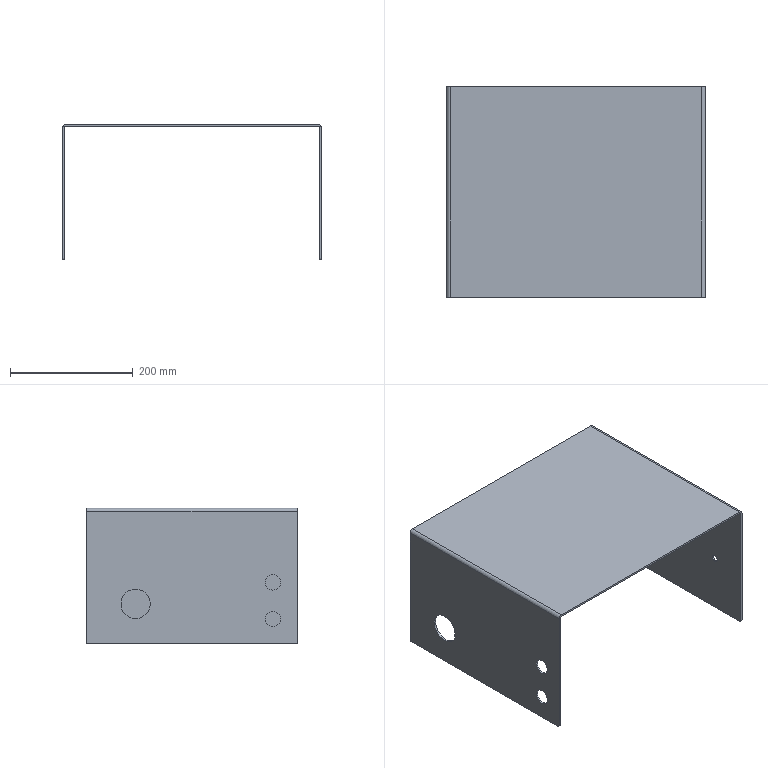Part | SolidWorks | features ICE 2, Fillet 1, FlatPattern 1, SMBaseFlange 1, SheetMetal 1, UnFold 1 | 1 solid | 36 faces | box 422 x 344 x 221 mm | volume 872945 mm3 | cylinder 18 | plane 18 | commonest cylinder face diameters 11 x6 6 x4 25 x4 5 x2 48 x2
STEP:
#1=CARTESIAN_POINT('',(-208.,92.,-180.));
#2=VERTEX_POINT('',#1);
#3=CARTESIAN_POINT('',(-208.,92.,-132.));
#4=VERTEX_POINT('',#3);
#5=CARTESIAN_POINT('',(-208.,92.,-156.));
#6=DIRECTION('',(-1.,0.,0.));
#7=DIRECTION('',(0.,0.,1.));
#8=AXIS2_PLACEMENT_3D('',#5,#6,#7);
#9=CIRCLE('',#8,24.);
#10=EDGE_CURVE('',#2,#4,#9,.T.);
#11=ORIENTED_EDGE('',*,*,#10,.F.);
#12=CARTESIAN_POINT('',(-211.,92.,-180.));
#13=VERTEX_POINT('',#12);
#14=CARTESIAN_POINT('',(-208.,92.,-180.));
#15=DIRECTION('',(-1.,0.,0.));
#16=VECTOR('',#15,1000.);
#17=LINE('',#14,#16);
#18=EDGE_CURVE('',#2,#13,#17,.T.);
#19=ORIENTED_EDGE('',*,*,#18,.T.);
#20=CARTESIAN_POINT('',(-211.,92.,-132.));
#21=VERTEX_POINT('',#20);
#22=CARTESIAN_POINT('',(-211.,92.,-156.));
#23=DIRECTION('',(-1.,0.,0.));
#24=DIRECTION('',(0.,0.,1.));
#25=AXIS2_PLACEMENT_3D('',#22,#23,#24);
#26=CIRCLE('',#25,24.);
#27=EDGE_CURVE('',#13,#21,#26,.T.);
#28=ORIENTED_EDGE('',*,*,#27,.T.);
#29=CARTESIAN_POINT('',(-208.,92.,-132.));
#30=DIRECTION('',(-1.,0.,0.));
#31=VECTOR('',#30,1000.);
#32=LINE('',#29,#31);
#33=EDGE_CURVE('',#4,#21,#32,.T.);
#34=ORIENTED_EDGE('',*,*,#33,.F.);
#35=EDGE_LOOP('',(#11,#19,#28,#34));
#36=FACE_OUTER_BOUND('',#35,.T.);
#37=CARTESIAN_POINT('',(-208.,92.,-156.));
#38=DIRECTION('',(-1.,0.,0.));
#39=DIRECTION('',(0.,0.,1.));
#40=AXIS2_PLACEMENT_3D('',#37,#38,#39);
#41=CYLINDRICAL_SURFACE('',#40,24.);
#42=ADVANCED_FACE('',(#36),#41,.F.);
#43=CARTESIAN_POINT('',(-208.,-132.,-193.5));
#44=VERTEX_POINT('',#43);
#45=CARTESIAN_POINT('',(-208.,-132.,-168.5));
#46=VERTEX_POINT('',#45);
#47=CARTESIAN_POINT('',(-208.,-132.,-181.));
#48=DIRECTION('',(-1.,0.,0.));
#49=DIRECTION('',(0.,0.,1.));
#50=AXIS2_PLACEMENT_3D('',#47,#48,#49);
#51=CIRCLE('',#50,12.5);
#52=EDGE_CURVE('',#44,#46,#51,.T.);
#53=ORIENTED_EDGE('',*,*,#52,.F.);
#54=CARTESIAN_POINT('',(-211.,-132.,-193.5));
#55=VERTEX_POINT('',#54);
#56=CARTESIAN_POINT('',(-208.,-132.,-193.5));
#57=DIRECTION('',(-1.,0.,0.));
#58=VECTOR('',#57,1000.);
#59=LINE('',#56,#58);
#60=EDGE_CURVE('',#44,#55,#59,.T.);
#61=ORIENTED_EDGE('',*,*,#60,.T.);
#62=CARTESIAN_POINT('',(-211.,-132.,-168.5));
#63=VERTEX_POINT('',#62);
#64=CARTESIAN_POINT('',(-211.,-132.,-181.));
#65=DIRECTION('',(-1.,0.,0.));
#66=DIRECTION('',(0.,0.,1.));
#67=AXIS2_PLACEMENT_3D('',#64,#65,#66);
#68=CIRCLE('',#67,12.5);
#69=EDGE_CURVE('',#55,#63,#68,.T.);
#70=ORIENTED_EDGE('',*,*,#69,.T.);
#71=CARTESIAN_POINT('',(-208.,-132.,-168.5));
#72=DIRECTION('',(-1.,0.,0.));
#73=VECTOR('',#72,1000.);
#74=LINE('',#71,#73);
#75=EDGE_CURVE('',#46,#63,#74,.T.);
#76=ORIENTED_EDGE('',*,*,#75,.F.);
#77=EDGE_LOOP('',(#53,#61,#70,#76));
#78=FACE_OUTER_BOUND('',#77,.T.);
#79=CARTESIAN_POINT('',(-208.,-132.,-181.));
#80=DIRECTION('',(-1.,0.,0.));
#81=DIRECTION('',(0.,0.,1.));
#82=AXIS2_PLACEMENT_3D('',#79,#80,#81);
#83=CYLINDRICAL_SURFACE('',#82,12.5);
#84=ADVANCED_FACE('',(#78),#83,.F.);
#85=CARTESIAN_POINT('',(-208.,-132.,-133.5));
#86=VERTEX_POINT('',#85);
#87=CARTESIAN_POINT('',(-208.,-132.,-108.5));
#88=VERTEX_POINT('',#87);
#89=CARTESIAN_POINT('',(-208.,-132.,-121.));
#90=DIRECTION('',(-1.,0.,0.));
#91=DIRECTION('',(0.,0.,1.));
#92=AXIS2_PLACEMENT_3D('',#89,#90,#91);
#93=CIRCLE('',#92,12.5);
#94=EDGE_CURVE('',#86,#88,#93,.T.);
#95=ORIENTED_EDGE('',*,*,#94,.F.);
#96=CARTESIAN_POINT('',(-211.,-132.,-133.5));
#97=VERTEX_POINT('',#96);
#98=CARTESIAN_POINT('',(-208.,-132.,-133.5));
#99=DIRECTION('',(-1.,0.,0.));
#100=VECTOR('',#99,1000.);
#101=LINE('',#98,#100);
#102=EDGE_CURVE('',#86,#97,#101,.T.);
#103=ORIENTED_EDGE('',*,*,#102,.T.);
#104=CARTESIAN_POINT('',(-211.,-132.,-108.5));
#105=VERTEX_POINT('',#104);
#106=CARTESIAN_POINT('',(-211.,-132.,-121.));
#107=DIRECTION('',(-1.,0.,0.));
#108=DIRECTION('',(0.,0.,1.));
#109=AXIS2_PLACEMENT_3D('',#106,#107,#108);
#110=CIRCLE('',#109,12.5);
#111=EDGE_CURVE('',#97,#105,#110,.T.);
#112=ORIENTED_EDGE('',*,*,#111,.T.);
#113=CARTESIAN_POINT('',(-208.,-132.,-108.5));
#114=DIRECTION('',(-1.,0.,0.));
#115=VECTOR('',#114,1000.);
#116=LINE('',#113,#115);
#117=EDGE_CURVE('',#88,#105,#116,.T.);
#118=ORIENTED_EDGE('',*,*,#117,.F.);
#119=EDGE_LOOP('',(#95,#103,#112,#118));
#120=FACE_OUTER_BOUND('',#119,.T.);
#121=CARTESIAN_POINT('',(-208.,-132.,-121.));
#122=DIRECTION('',(-1.,0.,0.));
#123=DIRECTION('',(0.,0.,1.));
#124=AXIS2_PLACEMENT_3D('',#121,#122,#123);
#125=CYLINDRICAL_SURFACE('',#124,12.5);
#126=ADVANCED_FACE('',(#120),#125,.F.);
#127=CARTESIAN_POINT('',(208.,-112.,-118.5));
#128=VERTEX_POINT('',#127);
#129=CARTESIAN_POINT('',(208.,-112.,-129.5));
#130=VERTEX_POINT('',#129);
#131=CARTESIAN_POINT('',(208.,-112.,-124.));
#132=DIRECTION('',(1.,0.,0.));
#133=DIRECTION('',(0.,0.,-1.));
#134=AXIS2_PLACEMENT_3D('',#131,#132,#133);
#135=CIRCLE('',#134,5.5);
#136=EDGE_CURVE('',#128,#130,#135,.T.);
#137=ORIENTED_EDGE('',*,*,#136,.F.);
#138=CARTESIAN_POINT('',(211.,-112.,-118.5));
#139=VERTEX_POINT('',#138);
#140=CARTESIAN_POINT('',(208.,-112.,-118.5));
#141=DIRECTION('',(1.,0.,0.));
#142=VECTOR('',#141,1000.);
#143=LINE('',#140,#142);
#144=EDGE_CURVE('',#128,#139,#143,.T.);
#145=ORIENTED_EDGE('',*,*,#144,.T.);
#146=CARTESIAN_POINT('',(211.,-112.,-129.5));
#147=VERTEX_POINT('',#146);
#148=CARTESIAN_POINT('',(211.,-112.,-124.));
#149=DIRECTION('',(1.,0.,0.));
#150=DIRECTION('',(0.,0.,-1.));
#151=AXIS2_PLACEMENT_3D('',#148,#149,#150);
#152=CIRCLE('',#151,5.5);
#153=EDGE_CURVE('',#139,#147,#152,.T.);
#154=ORIENTED_EDGE('',*,*,#153,.T.);
#155=CARTESIAN_POINT('',(208.,-112.,-129.5));
#156=DIRECTION('',(1.,0.,0.));
#157=VECTOR('',#156,1000.);
#158=LINE('',#155,#157);
#159=EDGE_CURVE('',#130,#147,#158,.T.);
#160=ORIENTED_EDGE('',*,*,#159,.F.);
#161=EDGE_LOOP('',(#137,#145,#154,#160));
#162=FACE_OUTER_BOUND('',#161,.T.);
#163=CARTESIAN_POINT('',(208.,-112.,-124.));
#164=DIRECTION('',(1.,0.,0.));
#165=DIRECTION('',(0.,0.,-1.));
#166=AXIS2_PLACEMENT_3D('',#163,#164,#165);
#167=CYLINDRICAL_SURFACE('',#166,5.5);
#168=ADVANCED_FACE('',(#162),#167,.F.);
#169=CARTESIAN_POINT('',(208.,38.,-118.5));
#170=VERTEX_POINT('',#169);
#171=CARTESIAN_POINT('',(208.,38.,-129.5));
#172=VERTEX_POINT('',#171);
#173=CARTESIAN_POINT('',(208.,38.,-124.));
#174=DIRECTION('',(1.,0.,0.));
#175=DIRECTION('',(0.,0.,-1.));
#176=AXIS2_PLACEMENT_3D('',#173,#174,#175);
#177=CIRCLE('',#176,5.5);
#178=EDGE_CURVE('',#170,#172,#177,.T.);
#179=ORIENTED_EDGE('',*,*,#178,.F.);
#180=CARTESIAN_POINT('',(211.,38.,-118.5));
#181=VERTEX_POINT('',#180);
#182=CARTESIAN_POINT('',(208.,38.,-118.5));
#183=DIRECTION('',(1.,0.,0.));
#184=VECTOR('',#183,1000.);
#185=LINE('',#182,#184);
#186=EDGE_CURVE('',#170,#181,#185,.T.);
#187=ORIENTED_EDGE('',*,*,#186,.T.);
#188=CARTESIAN_POINT('',(211.,38.,-129.5));
#189=VERTEX_POINT('',#188);
#190=CARTESIAN_POINT('',(211.,38.,-124.));
#191=DIRECTION('',(1.,0.,0.));
#192=DIRECTION('',(0.,0.,-1.));
#193=AXIS2_PLACEMENT_3D('',#190,#191,#192);
#194=CIRCLE('',#193,5.5);
#195=EDGE_CURVE('',#181,#189,#194,.T.);
#196=ORIENTED_EDGE('',*,*,#195,.T.);
#197=CARTESIAN_POINT('',(208.,38.,-129.5));
#198=DIRECTION('',(1.,0.,0.));
#199=VECTOR('',#198,1000.);
#200=LINE('',#197,#199);
#201=EDGE_CURVE('',#172,#189,#200,.T.);
#202=ORIENTED_EDGE('',*,*,#201,.F.);
#203=EDGE_LOOP('',(#179,#187,#196,#202));
#204=FACE_OUTER_BOUND('',#203,.T.);
#205=CARTESIAN_POINT('',(208.,38.,-124.));
#206=DIRECTION('',(1.,0.,0.));
#207=DIRECTION('',(0.,0.,-1.));
#208=AXIS2_PLACEMENT_3D('',#205,#206,#207);
#209=CYLINDRICAL_SURFACE('',#208,5.5);
#210=ADVANCED_FACE('',(#204),#209,.F.);
#211=CARTESIAN_POINT('',(205.5,172.,0.));
#212=VERTEX_POINT('',#211);
#213=CARTESIAN_POINT('',(205.5,172.,-3.));
#214=VERTEX_POINT('',#213);
#215=CARTESIAN_POINT('',(205.5,172.,0.));
#216=DIRECTION('',(0.,0.,-1.));
#217=VECTOR('',#216,1000.);
#218=LINE('',#215,#217);
#219=EDGE_CURVE('',#212,#214,#218,.T.);
#220=ORIENTED_EDGE('',*,*,#219,.F.);
#221=CARTESIAN_POINT('',(211.,172.,-5.5));
#222=VERTEX_POINT('',#221);
#223=CARTESIAN_POINT('',(205.5,172.,-5.5));
#224=DIRECTION('',(0.,-1.,0.));
#225=DIRECTION('',(0.,0.,1.));
#226=AXIS2_PLACEMENT_3D('',#223,#224,#225);
#227=CIRCLE('',#226,5.5);
#228=EDGE_CURVE('',#222,#212,#227,.T.);
#229=ORIENTED_EDGE('',*,*,#228,.F.);
#230=CARTESIAN_POINT('',(208.,172.,-5.5));
#231=VERTEX_POINT('',#230);
#232=CARTESIAN_POINT('',(208.,172.,-5.5));
#233=DIRECTION('',(1.,0.,0.));
#234=VECTOR('',#233,1000.);
#235=LINE('',#232,#234);
#236=EDGE_CURVE('',#231,#222,#235,.T.);
#237=ORIENTED_EDGE('',*,*,#236,.F.);
#238=CARTESIAN_POINT('',(205.5,172.,-5.5));
#239=DIRECTION('',(0.,-1.,0.));
#240=DIRECTION('',(1.,0.,0.));
#241=AXIS2_PLACEMENT_3D('',#238,#239,#240);
#242=CIRCLE('',#241,2.5);
#243=EDGE_CURVE('',#231,#214,#242,.T.);
#244=ORIENTED_EDGE('',*,*,#243,.T.);
#245=EDGE_LOOP('',(#220,#229,#237,#244));
#246=FACE_OUTER_BOUND('',#245,.T.);
#247=CARTESIAN_POINT('',(205.5,172.,0.));
#248=DIRECTION('',(0.,1.,0.));
#249=DIRECTION('',(0.,0.,1.));
#250=AXIS2_PLACEMENT_3D('',#247,#248,#249);
#251=PLANE('',#250);
#252=ADVANCED_FACE('',(#246),#251,.T.);
#253=CARTESIAN_POINT('',(-205.5,172.,0.));
#254=VERTEX_POINT('',#253);
#255=CARTESIAN_POINT('',(-211.,172.,0.));
#256=DIRECTION('',(-1.,0.,0.));
#257=VECTOR('',#256,1000.);
#258=LINE('',#255,#257);
#259=EDGE_CURVE('',#212,#254,#258,.T.);
#260=ORIENTED_EDGE('',*,*,#259,.F.);
#261=ORIENTED_EDGE('',*,*,#219,.T.);
#262=CARTESIAN_POINT('',(-205.5,172.,-3.));
#263=VERTEX_POINT('',#262);
#264=CARTESIAN_POINT('',(-211.,172.,-3.));
#265=DIRECTION('',(-1.,0.,0.));
#266=VECTOR('',#265,1000.);
#267=LINE('',#264,#266);
#268=EDGE_CURVE('',#214,#263,#267,.T.);
#269=ORIENTED_EDGE('',*,*,#268,.T.);
#270=CARTESIAN_POINT('',(-205.5,172.,-3.));
#271=DIRECTION('',(0.,0.,1.));
#272=VECTOR('',#271,1000.);
#273=LINE('',#270,#272);
#274=EDGE_CURVE('',#263,#254,#273,.T.);
#275=ORIENTED_EDGE('',*,*,#274,.T.);
#276=EDGE_LOOP('',(#260,#261,#269,#275));
#277=FACE_OUTER_BOUND('',#276,.T.);
#278=CARTESIAN_POINT('',(208.,172.,-5.5));
#279=DIRECTION('',(0.,1.,0.));
#280=DIRECTION('',(0.,0.,1.));
#281=AXIS2_PLACEMENT_3D('',#278,#279,#280);
#282=PLANE('',#281);
#283=ADVANCED_FACE('',(#277),#282,.T.);
#284=CARTESIAN_POINT('',(211.,-172.,-5.5));
#285=VERTEX_POINT('',#284);
#286=CARTESIAN_POINT('',(208.,-172.,-5.5));
#287=VERTEX_POINT('',#286);
#288=CARTESIAN_POINT('',(211.,-172.,-5.5));
#289=DIRECTION('',(-1.,0.,0.));
#290=VECTOR('',#289,1000.);
#291=LINE('',#288,#290);
#292=EDGE_CURVE('',#285,#287,#291,.T.);
#293=ORIENTED_EDGE('',*,*,#292,.F.);
#294=CARTESIAN_POINT('',(205.5,-172.,0.));
#295=VERTEX_POINT('',#294);
#296=CARTESIAN_POINT('',(205.5,-172.,-5.5));
#297=DIRECTION('',(0.,-1.,0.));
#298=DIRECTION('',(0.,0.,1.));
#299=AXIS2_PLACEMENT_3D('',#296,#297,#298);
#300=CIRCLE('',#299,5.5);
#301=EDGE_CURVE('',#285,#295,#300,.T.);
#302=ORIENTED_EDGE('',*,*,#301,.T.);
#303=CARTESIAN_POINT('',(205.5,-172.,-3.));
#304=VERTEX_POINT('',#303);
#305=CARTESIAN_POINT('',(205.5,-172.,-3.));
#306=DIRECTION('',(0.,0.,1.));
#307=VECTOR('',#306,1000.);
#308=LINE('',#305,#307);
#309=EDGE_CURVE('',#304,#295,#308,.T.);
#310=ORIENTED_EDGE('',*,*,#309,.F.);
#311=CARTESIAN_POINT('',(205.5,-172.,-5.5));
#312=DIRECTION('',(0.,-1.,0.));
#313=DIRECTION('',(1.,0.,0.));
#314=AXIS2_PLACEMENT_3D('',#311,#312,#313);
#315=CIRCLE('',#314,2.5);
#316=EDGE_CURVE('',#287,#304,#315,.T.);
#317=ORIENTED_EDGE('',*,*,#316,.F.);
#318=EDGE_LOOP('',(#293,#302,#310,#317));
#319=FACE_OUTER_BOUND('',#318,.T.);
#320=CARTESIAN_POINT('',(211.,-172.,-5.5));
#321=DIRECTION('',(0.,-1.,0.));
#322=DIRECTION('',(0.,0.,-1.));
#323=AXIS2_PLACEMENT_3D('',#320,#321,#322);
#324=PLANE('',#323);
#325=ADVANCED_FACE('',(#319),#324,.T.);
#326=CARTESIAN_POINT('',(208.,-172.,-218.));
#327=VERTEX_POINT('',#326);
#328=CARTESIAN_POINT('',(208.,-172.,0.));
#329=DIRECTION('',(0.,0.,1.));
#330=VECTOR('',#329,1000.);
#331=LINE('',#328,#330);
#332=EDGE_CURVE('',#327,#287,#331,.T.);
#333=ORIENTED_EDGE('',*,*,#332,.F.);
#334=CARTESIAN_POINT('',(211.,-172.,-218.));
#335=VERTEX_POINT('',#334);
#336=CARTESIAN_POINT('',(205.5,-172.,-218.));
#337=DIRECTION('',(1.,0.,0.));
#338=VECTOR('',#337,1000.);
#339=LINE('',#336,#338);
#340=EDGE_CURVE('',#327,#335,#339,.T.);
#341=ORIENTED_EDGE('',*,*,#340,.T.);
#342=CARTESIAN_POINT('',(211.,-172.,0.));
#343=DIRECTION('',(0.,0.,1.));
#344=VECTOR('',#343,1000.);
#345=LINE('',#342,#344);
#346=EDGE_CURVE('',#335,#285,#345,.T.);
#347=ORIENTED_EDGE('',*,*,#346,.T.);
#348=ORIENTED_EDGE('',*,*,#292,.T.);
#349=EDGE_LOOP('',(#333,#341,#347,#348));
#350=FACE_OUTER_BOUND('',#349,.T.);
#351=CARTESIAN_POINT('',(205.5,-172.,-3.));
#352=DIRECTION('',(0.,-1.,0.));
#353=DIRECTION('',(0.,0.,-1.));
#354=AXIS2_PLACEMENT_3D('',#351,#352,#353);
#355=PLANE('',#354);
#356=ADVANCED_FACE('',(#350),#355,.T.);
#357=CARTESIAN_POINT('',(-211.,172.,-5.5));
#358=VERTEX_POINT('',#357);
#359=CARTESIAN_POINT('',(-208.,172.,-5.5));
#360=VERTEX_POINT('',#359);
#361=CARTESIAN_POINT('',(-211.,172.,-5.5));
#362=DIRECTION('',(1.,0.,0.));
#363=VECTOR('',#362,1000.);
#364=LINE('',#361,#363);
#365=EDGE_CURVE('',#358,#360,#364,.T.);
#366=ORIENTED_EDGE('',*,*,#365,.F.);
#367=CARTESIAN_POINT('',(-205.5,172.,-5.5));
#368=DIRECTION('',(0.,-1.,0.));
#369=DIRECTION('',(0.,0.,1.));
#370=AXIS2_PLACEMENT_3D('',#367,#368,#369);
#371=CIRCLE('',#370,5.5);
#372=EDGE_CURVE('',#254,#358,#371,.T.);
#373=ORIENTED_EDGE('',*,*,#372,.F.);
#374=ORIENTED_EDGE('',*,*,#274,.F.);
#375=CARTESIAN_POINT('',(-205.5,172.,-5.5));
#376=DIRECTION('',(0.,-1.,0.));
#377=DIRECTION('',(1.,0.,0.));
#378=AXIS2_PLACEMENT_3D('',#375,#376,#377);
#379=CIRCLE('',#378,2.5);
#380=EDGE_CURVE('',#263,#360,#379,.T.);
#381=ORIENTED_EDGE('',*,*,#380,.T.);
#382=EDGE_LOOP('',(#366,#373,#374,#381));
#383=FACE_OUTER_BOUND('',#382,.T.);
#384=CARTESIAN_POINT('',(-211.,172.,-5.5));
#385=DIRECTION('',(0.,1.,0.));
#386=DIRECTION('',(0.,0.,1.));
#387=AXIS2_PLACEMENT_3D('',#384,#385,#386);
#388=PLANE('',#387);
#389=ADVANCED_FACE('',(#383),#388,.T.);
#390=CARTESIAN_POINT('',(-208.,172.,-218.));
#391=VERTEX_POINT('',#390);
#392=CARTESIAN_POINT('',(-208.,172.,0.));
#393=DIRECTION('',(0.,0.,-1.));
#394=VECTOR('',#393,1000.);
#395=LINE('',#392,#394);
#396=EDGE_CURVE('',#360,#391,#395,.T.);
#397=ORIENTED_EDGE('',*,*,#396,.T.);
#398=CARTESIAN_POINT('',(-211.,172.,-218.));
#399=VERTEX_POINT('',#398);
#400=CARTESIAN_POINT('',(-205.5,172.,-218.));
#401=DIRECTION('',(-1.,0.,0.));
#402=VECTOR('',#401,1000.);
#403=LINE('',#400,#402);
#404=EDGE_CURVE('',#391,#399,#403,.T.);
#405=ORIENTED_EDGE('',*,*,#404,.T.);
#406=CARTESIAN_POINT('',(-211.,172.,0.));
#407=DIRECTION('',(0.,0.,-1.));
#408=VECTOR('',#407,1000.);
#409=LINE('',#406,#408);
#410=EDGE_CURVE('',#358,#399,#409,.T.);
#411=ORIENTED_EDGE('',*,*,#410,.F.);
#412=ORIENTED_EDGE('',*,*,#365,.T.);
#413=EDGE_LOOP('',(#397,#405,#411,#412));
#414=FACE_OUTER_BOUND('',#413,.T.);
#415=CARTESIAN_POINT('',(-205.5,172.,-3.));
#416=DIRECTION('',(0.,1.,0.));
#417=DIRECTION('',(0.,0.,1.));
#418=AXIS2_PLACEMENT_3D('',#415,#416,#417);
#419=PLANE('',#418);
#420=ADVANCED_FACE('',(#414),#419,.T.);
#421=CARTESIAN_POINT('',(-205.5,-172.,0.));
#422=VERTEX_POINT('',#421);
#423=CARTESIAN_POINT('',(-205.5,-172.,-3.));
#424=VERTEX_POINT('',#423);
#425=CARTESIAN_POINT('',(-205.5,-172.,0.));
#426=DIRECTION('',(0.,0.,-1.));
#427=VECTOR('',#426,1000.);
#428=LINE('',#425,#427);
#429=EDGE_CURVE('',#422,#424,#428,.T.);
#430=ORIENTED_EDGE('',*,*,#429,.F.);
#431=CARTESIAN_POINT('',(-211.,-172.,-5.5));
#432=VERTEX_POINT('',#431);
#433=CARTESIAN_POINT('',(-205.5,-172.,-5.5));
#434=DIRECTION('',(0.,-1.,0.));
#435=DIRECTION('',(0.,0.,1.));
#436=AXIS2_PLACEMENT_3D('',#433,#434,#435);
#437=CIRCLE('',#436,5.5);
#438=EDGE_CURVE('',#422,#432,#437,.T.);
#439=ORIENTED_EDGE('',*,*,#438,.T.);
#440=CARTESIAN_POINT('',(-208.,-172.,-5.5));
#441=VERTEX_POINT('',#440);
#442=CARTESIAN_POINT('',(-208.,-172.,-5.5));
#443=DIRECTION('',(-1.,0.,0.));
#444=VECTOR('',#443,1000.);
#445=LINE('',#442,#444);
#446=EDGE_CURVE('',#441,#432,#445,.T.);
#447=ORIENTED_EDGE('',*,*,#446,.F.);
#448=CARTESIAN_POINT('',(-205.5,-172.,-5.5));
#449=DIRECTION('',(0.,-1.,0.));
#450=DIRECTION('',(1.,0.,0.));
#451=AXIS2_PLACEMENT_3D('',#448,#449,#450);
#452=CIRCLE('',#451,2.5);
#453=EDGE_CURVE('',#424,#441,#452,.T.);
#454=ORIENTED_EDGE('',*,*,#453,.F.);
#455=EDGE_LOOP('',(#430,#439,#447,#454));
#456=FACE_OUTER_BOUND('',#455,.T.);
#457=CARTESIAN_POINT('',(-205.5,-172.,0.));
#458=DIRECTION('',(0.,-1.,0.));
#459=DIRECTION('',(0.,0.,-1.));
#460=AXIS2_PLACEMENT_3D('',#457,#458,#459);
#461=PLANE('',#460);
#462=ADVANCED_FACE('',(#456),#461,.T.);
#463=CARTESIAN_POINT('',(-211.,-172.,0.));
#464=DIRECTION('',(-1.,0.,0.));
#465=VECTOR('',#464,1000.);
#466=LINE('',#463,#465);
#467=EDGE_CURVE('',#295,#422,#466,.T.);
#468=ORIENTED_EDGE('',*,*,#467,.T.);
#469=ORIENTED_EDGE('',*,*,#429,.T.);
#470=CARTESIAN_POINT('',(-211.,-172.,-3.));
#471=DIRECTION('',(-1.,0.,0.));
#472=VECTOR('',#471,1000.);
#473=LINE('',#470,#472);
#474=EDGE_CURVE('',#304,#424,#473,.T.);
#475=ORIENTED_EDGE('',*,*,#474,.F.);
#476=ORIENTED_EDGE('',*,*,#309,.T.);
#477=EDGE_LOOP('',(#468,#469,#475,#476));
#478=FACE_OUTER_BOUND('',#477,.T.);
#479=CARTESIAN_POINT('',(-208.,-172.,-5.5));
#480=DIRECTION('',(0.,-1.,0.));
#481=DIRECTION('',(0.,0.,-1.));
#482=AXIS2_PLACEMENT_3D('',#479,#480,#481);
#483=PLANE('',#482);
#484=ADVANCED_FACE('',(#478),#483,.T.);
#485=CARTESIAN_POINT('',(-208.,92.,-156.));
#486=DIRECTION('',(-1.,0.,0.));
#487=DIRECTION('',(0.,0.,1.));
#488=AXIS2_PLACEMENT_3D('',#485,#486,#487);
#489=CIRCLE('',#488,24.);
#490=EDGE_CURVE('',#4,#2,#489,.T.);
#491=ORIENTED_EDGE('',*,*,#490,.T.);
#492=ORIENTED_EDGE('',*,*,#10,.T.);
#493=EDGE_LOOP('',(#491,#492));
#494=FACE_BOUND('',#493,.T.);
#495=CARTESIAN_POINT('',(-208.,-132.,-181.));
#496=DIRECTION('',(-1.,0.,0.));
#497=DIRECTION('',(0.,0.,1.));
#498=AXIS2_PLACEMENT_3D('',#495,#496,#497);
#499=CIRCLE('',#498,12.5);
#500=EDGE_CURVE('',#46,#44,#499,.T.);
#501=ORIENTED_EDGE('',*,*,#500,.T.);
#502=ORIENTED_EDGE('',*,*,#52,.T.);
#503=EDGE_LOOP('',(#501,#502));
#504=FACE_BOUND('',#503,.T.);
#505=CARTESIAN_POINT('',(-208.,-132.,-121.));
#506=DIRECTION('',(-1.,0.,0.));
#507=DIRECTION('',(0.,0.,1.));
#508=AXIS2_PLACEMENT_3D('',#505,#506,#507);
#509=CIRCLE('',#508,12.5);
#510=EDGE_CURVE('',#88,#86,#509,.T.);
#511=ORIENTED_EDGE('',*,*,#510,.T.);
#512=ORIENTED_EDGE('',*,*,#94,.T.);
#513=EDGE_LOOP('',(#511,#512));
#514=FACE_BOUND('',#513,.T.);
#515=CARTESIAN_POINT('',(-208.,169.,-221.));
#516=VERTEX_POINT('',#515);
#517=CARTESIAN_POINT('',(-208.,-169.,-221.));
#518=VERTEX_POINT('',#517);
#519=CARTESIAN_POINT('',(-208.,172.,-221.));
#520=DIRECTION('',(0.,-1.,0.));
#521=VECTOR('',#520,1000.);
#522=LINE('',#519,#521);
#523=EDGE_CURVE('',#516,#518,#522,.T.);
#524=ORIENTED_EDGE('',*,*,#523,.F.);
#525=CARTESIAN_POINT('',(-208.,169.,-218.));
#526=DIRECTION('',(1.,0.,0.));
#527=DIRECTION('',(0.,0.,1.));
#528=AXIS2_PLACEMENT_3D('',#525,#526,#527);
#529=CIRCLE('',#528,3.);
#530=EDGE_CURVE('',#516,#391,#529,.T.);
#531=ORIENTED_EDGE('',*,*,#530,.T.);
#532=ORIENTED_EDGE('',*,*,#396,.F.);
#533=CARTESIAN_POINT('',(-208.,172.,-5.5));
#534=DIRECTION('',(0.,-1.,0.));
#535=VECTOR('',#534,1000.);
#536=LINE('',#533,#535);
#537=EDGE_CURVE('',#360,#441,#536,.T.);
#538=ORIENTED_EDGE('',*,*,#537,.T.);
#539=CARTESIAN_POINT('',(-208.,-172.,-218.));
#540=VERTEX_POINT('',#539);
#541=CARTESIAN_POINT('',(-208.,-172.,0.));
#542=DIRECTION('',(0.,0.,-1.));
#543=VECTOR('',#542,1000.);
#544=LINE('',#541,#543);
#545=EDGE_CURVE('',#441,#540,#544,.T.);
#546=ORIENTED_EDGE('',*,*,#545,.T.);
#547=CARTESIAN_POINT('',(-208.,-169.,-218.));
#548=DIRECTION('',(1.,0.,0.));
#549=DIRECTION('',(0.,0.,1.));
#550=AXIS2_PLACEMENT_3D('',#547,#548,#549);
#551=CIRCLE('',#550,3.);
#552=EDGE_CURVE('',#540,#518,#551,.T.);
#553=ORIENTED_EDGE('',*,*,#552,.T.);
#554=EDGE_LOOP('',(#524,#531,#532,#538,#546,#553));
#555=FACE_OUTER_BOUND('',#554,.T.);
#556=CARTESIAN_POINT('',(-208.,172.,0.));
#557=DIRECTION('',(-1.,0.,0.));
#558=DIRECTION('',(0.,0.,1.));
#559=AXIS2_PLACEMENT_3D('',#556,#557,#558);
#560=PLANE('',#559);
#561=ADVANCED_FACE('',(#494,#504,#514,#555),#560,.F.);
#562=CARTESIAN_POINT('',(-211.,169.,-221.));
#563=VERTEX_POINT('',#562);
#564=CARTESIAN_POINT('',(-211.,-169.,-221.));
#565=VERTEX_POINT('',#564);
#566=CARTESIAN_POINT('',(-211.,172.,-221.));
#567=DIRECTION('',(0.,-1.,0.));
#568=VECTOR('',#567,1000.);
#569=LINE('',#566,#568);
#570=EDGE_CURVE('',#563,#565,#569,.T.);
#571=ORIENTED_EDGE('',*,*,#570,.F.);
#572=CARTESIAN_POINT('',(-211.,169.,-221.));
#573=DIRECTION('',(1.,0.,0.));
#574=VECTOR('',#573,1000.);
#575=LINE('',#572,#574);
#576=EDGE_CURVE('',#563,#516,#575,.T.);
#577=ORIENTED_EDGE('',*,*,#576,.T.);
#578=ORIENTED_EDGE('',*,*,#523,.T.);
#579=CARTESIAN_POINT('',(-211.,-169.,-221.));
#580=DIRECTION('',(-1.,0.,0.));
#581=VECTOR('',#580,1000.);
#582=LINE('',#579,#581);
#583=EDGE_CURVE('',#518,#565,#582,.T.);
#584=ORIENTED_EDGE('',*,*,#583,.T.);
#585=EDGE_LOOP('',(#571,#577,#578,#584));
#586=FACE_OUTER_BOUND('',#585,.T.);
#587=CARTESIAN_POINT('',(-211.,172.,-221.));
#588=DIRECTION('',(0.,0.,-1.));
#589=DIRECTION('',(-1.,0.,0.));
#590=AXIS2_PLACEMENT_3D('',#587,#588,#589);
#591=PLANE('',#590);
#592=ADVANCED_FACE('',(#586),#591,.T.);
#593=CARTESIAN_POINT('',(-211.,92.,-156.));
#594=DIRECTION('',(-1.,0.,0.));
#595=DIRECTION('',(0.,0.,1.));
#596=AXIS2_PLACEMENT_3D('',#593,#594,#595);
#597=CIRCLE('',#596,24.);
#598=EDGE_CURVE('',#21,#13,#597,.T.);
#599=ORIENTED_EDGE('',*,*,#598,.F.);
#600=ORIENTED_EDGE('',*,*,#27,.F.);
#601=EDGE_LOOP('',(#599,#600));
#602=FACE_BOUND('',#601,.T.);
#603=CARTESIAN_POINT('',(-211.,-132.,-181.));
#604=DIRECTION('',(-1.,0.,0.));
#605=DIRECTION('',(0.,0.,1.));
#606=AXIS2_PLACEMENT_3D('',#603,#604,#605);
#607=CIRCLE('',#606,12.5);
#608=EDGE_CURVE('',#63,#55,#607,.T.);
#609=ORIENTED_EDGE('',*,*,#608,.F.);
#610=ORIENTED_EDGE('',*,*,#69,.F.);
#611=EDGE_LOOP('',(#609,#610));
#612=FACE_BOUND('',#611,.T.);
#613=CARTESIAN_POINT('',(-211.,-132.,-121.));
#614=DIRECTION('',(-1.,0.,0.));
#615=DIRECTION('',(0.,0.,1.));
#616=AXIS2_PLACEMENT_3D('',#613,#614,#615);
#617=CIRCLE('',#616,12.5);
#618=EDGE_CURVE('',#105,#97,#617,.T.);
#619=ORIENTED_EDGE('',*,*,#618,.F.);
#620=ORIENTED_EDGE('',*,*,#111,.F.);
#621=EDGE_LOOP('',(#619,#620));
#622=FACE_BOUND('',#621,.T.);
#623=ORIENTED_EDGE('',*,*,#410,.T.);
#624=CARTESIAN_POINT('',(-211.,169.,-218.));
#625=DIRECTION('',(-1.,0.,0.));
#626=DIRECTION('',(0.,0.,1.));
#627=AXIS2_PLACEMENT_3D('',#624,#625,#626);
#628=CIRCLE('',#627,3.);
#629=EDGE_CURVE('',#399,#563,#628,.T.);
#630=ORIENTED_EDGE('',*,*,#629,.T.);
#631=ORIENTED_EDGE('',*,*,#570,.T.);
#632=CARTESIAN_POINT('',(-211.,-172.,-218.));
#633=VERTEX_POINT('',#632);
#634=CARTESIAN_POINT('',(-211.,-169.,-218.));
#635=DIRECTION('',(-1.,0.,0.));
#636=DIRECTION('',(0.,0.,1.));
#637=AXIS2_PLACEMENT_3D('',#634,#635,#636);
#638=CIRCLE('',#637,3.);
#639=EDGE_CURVE('',#565,#633,#638,.T.);
#640=ORIENTED_EDGE('',*,*,#639,.T.);
#641=CARTESIAN_POINT('',(-211.,-172.,0.));
#642=DIRECTION('',(0.,0.,-1.));
#643=VECTOR('',#642,1000.);
#644=LINE('',#641,#643);
#645=EDGE_CURVE('',#432,#633,#644,.T.);
#646=ORIENTED_EDGE('',*,*,#645,.F.);
#647=CARTESIAN_POINT('',(-211.,172.,-5.5));
#648=DIRECTION('',(0.,-1.,0.));
#649=VECTOR('',#648,1000.);
#650=LINE('',#647,#649);
#651=EDGE_CURVE('',#358,#432,#650,.T.);
#652=ORIENTED_EDGE('',*,*,#651,.F.);
#653=EDGE_LOOP('',(#623,#630,#631,#640,#646,#652));
#654=FACE_OUTER_BOUND('',#653,.T.);
#655=CARTESIAN_POINT('',(-211.,172.,0.));
#656=DIRECTION('',(-1.,0.,0.));
#657=DIRECTION('',(0.,0.,1.));
#658=AXIS2_PLACEMENT_3D('',#655,#656,#657);
#659=PLANE('',#658);
#660=ADVANCED_FACE('',(#602,#612,#622,#654),#659,.T.);
#661=ORIENTED_EDGE('',*,*,#438,.F.);
#662=CARTESIAN_POINT('',(-205.5,172.,0.));
#663=DIRECTION('',(0.,-1.,0.));
#664=VECTOR('',#663,1000.);
#665=LINE('',#662,#664);
#666=EDGE_CURVE('',#254,#422,#665,.T.);
#667=ORIENTED_EDGE('',*,*,#666,.F.);
#668=ORIENTED_EDGE('',*,*,#372,.T.);
#669=ORIENTED_EDGE('',*,*,#651,.T.);
#670=EDGE_LOOP('',(#661,#667,#668,#669));
#671=FACE_OUTER_BOUND('',#670,.T.);
#672=CARTESIAN_POINT('',(-205.5,172.,-5.5));
#673=DIRECTION('',(0.,-1.,0.));
#674=DIRECTION('',(0.,0.,-1.));
#675=AXIS2_PLACEMENT_3D('',#672,#673,#674);
#676=CYLINDRICAL_SURFACE('',#675,5.5);
#677=ADVANCED_FACE('',(#671),#676,.T.);
#678=ORIENTED_EDGE('',*,*,#467,.F.);
#679=CARTESIAN_POINT('',(205.5,172.,0.));
#680=DIRECTION('',(0.,-1.,0.));
#681=VECTOR('',#680,1000.);
#682=LINE('',#679,#681);
#683=EDGE_CURVE('',#212,#295,#682,.T.);
#684=ORIENTED_EDGE('',*,*,#683,.F.);
#685=ORIENTED_EDGE('',*,*,#259,.T.);
#686=ORIENTED_EDGE('',*,*,#666,.T.);
#687=EDGE_LOOP('',(#678,#684,#685,#686));
#688=FACE_OUTER_BOUND('',#687,.T.);
#689=CARTESIAN_POINT('',(-211.,172.,0.));
#690=DIRECTION('',(0.,0.,1.));
#691=DIRECTION('',(1.,0.,0.));
#692=AXIS2_PLACEMENT_3D('',#689,#690,#691);
#693=PLANE('',#692);
#694=ADVANCED_FACE('',(#688),#693,.T.);
#695=ORIENTED_EDGE('',*,*,#301,.F.);
#696=CARTESIAN_POINT('',(211.,172.,-5.5));
#697=DIRECTION('',(0.,-1.,0.));
#698=VECTOR('',#697,1000.);
#699=LINE('',#696,#698);
#700=EDGE_CURVE('',#222,#285,#699,.T.);
#701=ORIENTED_EDGE('',*,*,#700,.F.);
#702=ORIENTED_EDGE('',*,*,#228,.T.);
#703=ORIENTED_EDGE('',*,*,#683,.T.);
#704=EDGE_LOOP('',(#695,#701,#702,#703));
#705=FACE_OUTER_BOUND('',#704,.T.);
#706=CARTESIAN_POINT('',(205.5,172.,-5.5));
#707=DIRECTION('',(0.,-1.,0.));
#708=DIRECTION('',(0.,0.,-1.));
#709=AXIS2_PLACEMENT_3D('',#706,#707,#708);
#710=CYLINDRICAL_SURFACE('',#709,5.5);
#711=ADVANCED_FACE('',(#705),#710,.T.);
#712=CARTESIAN_POINT('',(211.,-112.,-124.));
#713=DIRECTION('',(1.,0.,0.));
#714=DIRECTION('',(0.,0.,-1.));
#715=AXIS2_PLACEMENT_3D('',#712,#713,#714);
#716=CIRCLE('',#715,5.5);
#717=EDGE_CURVE('',#147,#139,#716,.T.);
#718=ORIENTED_EDGE('',*,*,#717,.F.);
#719=ORIENTED_EDGE('',*,*,#153,.F.);
#720=EDGE_LOOP('',(#718,#719));
#721=FACE_BOUND('',#720,.T.);
#722=CARTESIAN_POINT('',(211.,38.,-124.));
#723=DIRECTION('',(1.,0.,0.));
#724=DIRECTION('',(0.,0.,-1.));
#725=AXIS2_PLACEMENT_3D('',#722,#723,#724);
#726=CIRCLE('',#725,5.5);
#727=EDGE_CURVE('',#189,#181,#726,.T.);
#728=ORIENTED_EDGE('',*,*,#727,.F.);
#729=ORIENTED_EDGE('',*,*,#195,.F.);
#730=EDGE_LOOP('',(#728,#729));
#731=FACE_BOUND('',#730,.T.);
#732=ORIENTED_EDGE('',*,*,#346,.F.);
#733=CARTESIAN_POINT('',(211.,-169.,-221.));
#734=VERTEX_POINT('',#733);
#735=CARTESIAN_POINT('',(211.,-169.,-218.));
#736=DIRECTION('',(1.,0.,0.));
#737=DIRECTION('',(0.,0.,-1.));
#738=AXIS2_PLACEMENT_3D('',#735,#736,#737);
#739=CIRCLE('',#738,3.);
#740=EDGE_CURVE('',#335,#734,#739,.T.);
#741=ORIENTED_EDGE('',*,*,#740,.T.);
#742=CARTESIAN_POINT('',(211.,169.,-221.));
#743=VERTEX_POINT('',#742);
#744=CARTESIAN_POINT('',(211.,172.,-221.));
#745=DIRECTION('',(0.,-1.,0.));
#746=VECTOR('',#745,1000.);
#747=LINE('',#744,#746);
#748=EDGE_CURVE('',#743,#734,#747,.T.);
#749=ORIENTED_EDGE('',*,*,#748,.F.);
#750=CARTESIAN_POINT('',(211.,172.,-218.));
#751=VERTEX_POINT('',#750);
#752=CARTESIAN_POINT('',(211.,169.,-218.));
#753=DIRECTION('',(1.,0.,0.));
#754=DIRECTION('',(0.,0.,-1.));
#755=AXIS2_PLACEMENT_3D('',#752,#753,#754);
#756=CIRCLE('',#755,3.);
#757=EDGE_CURVE('',#743,#751,#756,.T.);
#758=ORIENTED_EDGE('',*,*,#757,.T.);
#759=CARTESIAN_POINT('',(211.,172.,0.));
#760=DIRECTION('',(0.,0.,1.));
#761=VECTOR('',#760,1000.);
#762=LINE('',#759,#761);
#763=EDGE_CURVE('',#751,#222,#762,.T.);
#764=ORIENTED_EDGE('',*,*,#763,.T.);
#765=ORIENTED_EDGE('',*,*,#700,.T.);
#766=EDGE_LOOP('',(#732,#741,#749,#758,#764,#765));
#767=FACE_OUTER_BOUND('',#766,.T.);
#768=CARTESIAN_POINT('',(211.,172.,0.));
#769=DIRECTION('',(1.,0.,0.));
#770=DIRECTION('',(0.,0.,-1.));
#771=AXIS2_PLACEMENT_3D('',#768,#769,#770);
#772=PLANE('',#771);
#773=ADVANCED_FACE('',(#721,#731,#767),#772,.T.);
#774=ORIENTED_EDGE('',*,*,#748,.T.);
#775=CARTESIAN_POINT('',(208.,-169.,-221.));
#776=VERTEX_POINT('',#775);
#777=CARTESIAN_POINT('',(208.,-169.,-221.));
#778=DIRECTION('',(-1.,0.,0.));
#779=VECTOR('',#778,1000.);
#780=LINE('',#777,#779);
#781=EDGE_CURVE('',#734,#776,#780,.T.);
#782=ORIENTED_EDGE('',*,*,#781,.T.);
#783=CARTESIAN_POINT('',(208.,169.,-221.));
#784=VERTEX_POINT('',#783);
#785=CARTESIAN_POINT('',(208.,172.,-221.));
#786=DIRECTION('',(0.,-1.,0.));
#787=VECTOR('',#786,1000.);
#788=LINE('',#785,#787);
#789=EDGE_CURVE('',#784,#776,#788,.T.);
#790=ORIENTED_EDGE('',*,*,#789,.F.);
#791=CARTESIAN_POINT('',(208.,169.,-221.));
#792=DIRECTION('',(1.,0.,0.));
#793=VECTOR('',#792,1000.);
#794=LINE('',#791,#793);
#795=EDGE_CURVE('',#784,#743,#794,.T.);
#796=ORIENTED_EDGE('',*,*,#795,.T.);
#797=EDGE_LOOP('',(#774,#782,#790,#796));
#798=FACE_OUTER_BOUND('',#797,.T.);
#799=CARTESIAN_POINT('',(208.,172.,-221.));
#800=DIRECTION('',(0.,0.,-1.));
#801=DIRECTION('',(-1.,0.,0.));
#802=AXIS2_PLACEMENT_3D('',#799,#800,#801);
#803=PLANE('',#802);
#804=ADVANCED_FACE('',(#798),#803,.T.);
#805=CARTESIAN_POINT('',(208.,-112.,-124.));
#806=DIRECTION('',(1.,0.,0.));
#807=DIRECTION('',(0.,0.,-1.));
#808=AXIS2_PLACEMENT_3D('',#805,#806,#807);
#809=CIRCLE('',#808,5.5);
#810=EDGE_CURVE('',#130,#128,#809,.T.);
#811=ORIENTED_EDGE('',*,*,#810,.T.);
#812=ORIENTED_EDGE('',*,*,#136,.T.);
#813=EDGE_LOOP('',(#811,#812));
#814=FACE_BOUND('',#813,.T.);
#815=CARTESIAN_POINT('',(208.,38.,-124.));
#816=DIRECTION('',(1.,0.,0.));
#817=DIRECTION('',(0.,0.,-1.));
#818=AXIS2_PLACEMENT_3D('',#815,#816,#817);
#819=CIRCLE('',#818,5.5);
#820=EDGE_CURVE('',#172,#170,#819,.T.);
#821=ORIENTED_EDGE('',*,*,#820,.T.);
#822=ORIENTED_EDGE('',*,*,#178,.T.);
#823=EDGE_LOOP('',(#821,#822));
#824=FACE_BOUND('',#823,.T.);
#825=ORIENTED_EDGE('',*,*,#789,.T.);
#826=CARTESIAN_POINT('',(208.,-169.,-218.));
#827=DIRECTION('',(-1.,0.,0.));
#828=DIRECTION('',(0.,0.,-1.));
#829=AXIS2_PLACEMENT_3D('',#826,#827,#828);
#830=CIRCLE('',#829,3.);
#831=EDGE_CURVE('',#776,#327,#830,.T.);
#832=ORIENTED_EDGE('',*,*,#831,.T.);
#833=ORIENTED_EDGE('',*,*,#332,.T.);
#834=CARTESIAN_POINT('',(208.,172.,-5.5));
#835=DIRECTION('',(0.,-1.,0.));
#836=VECTOR('',#835,1000.);
#837=LINE('',#834,#836);
#838=EDGE_CURVE('',#231,#287,#837,.T.);
#839=ORIENTED_EDGE('',*,*,#838,.F.);
#840=CARTESIAN_POINT('',(208.,172.,-218.));
#841=VERTEX_POINT('',#840);
#842=CARTESIAN_POINT('',(208.,172.,0.));
#843=DIRECTION('',(0.,0.,1.));
#844=VECTOR('',#843,1000.);
#845=LINE('',#842,#844);
#846=EDGE_CURVE('',#841,#231,#845,.T.);
#847=ORIENTED_EDGE('',*,*,#846,.F.);
#848=CARTESIAN_POINT('',(208.,169.,-218.));
#849=DIRECTION('',(-1.,0.,0.));
#850=DIRECTION('',(0.,0.,-1.));
#851=AXIS2_PLACEMENT_3D('',#848,#849,#850);
#852=CIRCLE('',#851,3.);
#853=EDGE_CURVE('',#841,#784,#852,.T.);
#854=ORIENTED_EDGE('',*,*,#853,.T.);
#855=EDGE_LOOP('',(#825,#832,#833,#839,#847,#854));
#856=FACE_OUTER_BOUND('',#855,.T.);
#857=CARTESIAN_POINT('',(208.,172.,0.));
#858=DIRECTION('',(1.,0.,0.));
#859=DIRECTION('',(0.,0.,-1.));
#860=AXIS2_PLACEMENT_3D('',#857,#858,#859);
#861=PLANE('',#860);
#862=ADVANCED_FACE('',(#814,#824,#856),#861,.F.);
#863=ORIENTED_EDGE('',*,*,#316,.T.);
#864=CARTESIAN_POINT('',(205.5,172.,-3.));
#865=DIRECTION('',(0.,-1.,0.));
#866=VECTOR('',#865,1000.);
#867=LINE('',#864,#866);
#868=EDGE_CURVE('',#214,#304,#867,.T.);
#869=ORIENTED_EDGE('',*,*,#868,.F.);
#870=ORIENTED_EDGE('',*,*,#243,.F.);
#871=ORIENTED_EDGE('',*,*,#838,.T.);
#872=EDGE_LOOP('',(#863,#869,#870,#871));
#873=FACE_OUTER_BOUND('',#872,.T.);
#874=CARTESIAN_POINT('',(205.5,172.,-5.5));
#875=DIRECTION('',(0.,-1.,0.));
#876=DIRECTION('',(0.,0.,-1.));
#877=AXIS2_PLACEMENT_3D('',#874,#875,#876);
#878=CYLINDRICAL_SURFACE('',#877,2.5);
#879=ADVANCED_FACE('',(#873),#878,.F.);
#880=ORIENTED_EDGE('',*,*,#474,.T.);
#881=CARTESIAN_POINT('',(-205.5,172.,-3.));
#882=DIRECTION('',(0.,-1.,0.));
#883=VECTOR('',#882,1000.);
#884=LINE('',#881,#883);
#885=EDGE_CURVE('',#263,#424,#884,.T.);
#886=ORIENTED_EDGE('',*,*,#885,.F.);
#887=ORIENTED_EDGE('',*,*,#268,.F.);
#888=ORIENTED_EDGE('',*,*,#868,.T.);
#889=EDGE_LOOP('',(#880,#886,#887,#888));
#890=FACE_OUTER_BOUND('',#889,.T.);
#891=CARTESIAN_POINT('',(-211.,172.,-3.));
#892=DIRECTION('',(0.,0.,1.));
#893=DIRECTION('',(1.,0.,0.));
#894=AXIS2_PLACEMENT_3D('',#891,#892,#893);
#895=PLANE('',#894);
#896=ADVANCED_FACE('',(#890),#895,.F.);
#897=ORIENTED_EDGE('',*,*,#453,.T.);
#898=ORIENTED_EDGE('',*,*,#537,.F.);
#899=ORIENTED_EDGE('',*,*,#380,.F.);
#900=ORIENTED_EDGE('',*,*,#885,.T.);
#901=EDGE_LOOP('',(#897,#898,#899,#900));
#902=FACE_OUTER_BOUND('',#901,.T.);
#903=CARTESIAN_POINT('',(-205.5,172.,-5.5));
#904=DIRECTION('',(0.,-1.,0.));
#905=DIRECTION('',(0.,0.,-1.));
#906=AXIS2_PLACEMENT_3D('',#903,#904,#905);
#907=CYLINDRICAL_SURFACE('',#906,2.5);
#908=ADVANCED_FACE('',(#902),#907,.F.);
#909=ORIENTED_EDGE('',*,*,#763,.F.);
#910=CARTESIAN_POINT('',(-205.5,172.,-218.));
#911=DIRECTION('',(-1.,0.,0.));
#912=VECTOR('',#911,1000.);
#913=LINE('',#910,#912);
#914=EDGE_CURVE('',#751,#841,#913,.T.);
#915=ORIENTED_EDGE('',*,*,#914,.T.);
#916=ORIENTED_EDGE('',*,*,#846,.T.);
#917=ORIENTED_EDGE('',*,*,#236,.T.);
#918=EDGE_LOOP('',(#909,#915,#916,#917));
#919=FACE_OUTER_BOUND('',#918,.T.);
#920=CARTESIAN_POINT('',(-205.5,172.,-5.5));
#921=DIRECTION('',(0.,1.,0.));
#922=DIRECTION('',(1.,0.,0.));
#923=AXIS2_PLACEMENT_3D('',#920,#921,#922);
#924=PLANE('',#923);
#925=ADVANCED_FACE('',(#919),#924,.T.);
#926=ORIENTED_EDGE('',*,*,#645,.T.);
#927=CARTESIAN_POINT('',(-208.,-172.,-218.));
#928=DIRECTION('',(1.,0.,0.));
#929=VECTOR('',#928,1000.);
#930=LINE('',#927,#929);
#931=EDGE_CURVE('',#633,#540,#930,.T.);
#932=ORIENTED_EDGE('',*,*,#931,.T.);
#933=ORIENTED_EDGE('',*,*,#545,.F.);
#934=ORIENTED_EDGE('',*,*,#446,.T.);
#935=EDGE_LOOP('',(#926,#932,#933,#934));
#936=FACE_OUTER_BOUND('',#935,.T.);
#937=CARTESIAN_POINT('',(-205.5,-172.,-5.5));
#938=DIRECTION('',(0.,1.,0.));
#939=DIRECTION('',(1.,0.,0.));
#940=AXIS2_PLACEMENT_3D('',#937,#938,#939);
#941=PLANE('',#940);
#942=ADVANCED_FACE('',(#936),#941,.F.);
#943=ORIENTED_EDGE('',*,*,#186,.F.);
#944=ORIENTED_EDGE('',*,*,#820,.F.);
#945=ORIENTED_EDGE('',*,*,#201,.T.);
#946=ORIENTED_EDGE('',*,*,#727,.T.);
#947=EDGE_LOOP('',(#943,#944,#945,#946));
#948=FACE_OUTER_BOUND('',#947,.T.);
#949=CARTESIAN_POINT('',(208.,38.,-124.));
#950=DIRECTION('',(1.,0.,0.));
#951=DIRECTION('',(0.,0.,-1.));
#952=AXIS2_PLACEMENT_3D('',#949,#950,#951);
#953=CYLINDRICAL_SURFACE('',#952,5.5);
#954=ADVANCED_FACE('',(#948),#953,.F.);
#955=ORIENTED_EDGE('',*,*,#144,.F.);
#956=ORIENTED_EDGE('',*,*,#810,.F.);
#957=ORIENTED_EDGE('',*,*,#159,.T.);
#958=ORIENTED_EDGE('',*,*,#717,.T.);
#959=EDGE_LOOP('',(#955,#956,#957,#958));
#960=FACE_OUTER_BOUND('',#959,.T.);
#961=CARTESIAN_POINT('',(208.,-112.,-124.));
#962=DIRECTION('',(1.,0.,0.));
#963=DIRECTION('',(0.,0.,-1.));
#964=AXIS2_PLACEMENT_3D('',#961,#962,#963);
#965=CYLINDRICAL_SURFACE('',#964,5.5);
#966=ADVANCED_FACE('',(#960),#965,.F.);
#967=ORIENTED_EDGE('',*,*,#102,.F.);
#968=ORIENTED_EDGE('',*,*,#510,.F.);
#969=ORIENTED_EDGE('',*,*,#117,.T.);
#970=ORIENTED_EDGE('',*,*,#618,.T.);
#971=EDGE_LOOP('',(#967,#968,#969,#970));
#972=FACE_OUTER_BOUND('',#971,.T.);
#973=CARTESIAN_POINT('',(-208.,-132.,-121.));
#974=DIRECTION('',(-1.,0.,0.));
#975=DIRECTION('',(0.,0.,1.));
#976=AXIS2_PLACEMENT_3D('',#973,#974,#975);
#977=CYLINDRICAL_SURFACE('',#976,12.5);
#978=ADVANCED_FACE('',(#972),#977,.F.);
#979=ORIENTED_EDGE('',*,*,#60,.F.);
#980=ORIENTED_EDGE('',*,*,#500,.F.);
#981=ORIENTED_EDGE('',*,*,#75,.T.);
#982=ORIENTED_EDGE('',*,*,#608,.T.);
#983=EDGE_LOOP('',(#979,#980,#981,#982));
#984=FACE_OUTER_BOUND('',#983,.T.);
#985=CARTESIAN_POINT('',(-208.,-132.,-181.));
#986=DIRECTION('',(-1.,0.,0.));
#987=DIRECTION('',(0.,0.,1.));
#988=AXIS2_PLACEMENT_3D('',#985,#986,#987);
#989=CYLINDRICAL_SURFACE('',#988,12.5);
#990=ADVANCED_FACE('',(#984),#989,.F.);
#991=ORIENTED_EDGE('',*,*,#18,.F.);
#992=ORIENTED_EDGE('',*,*,#490,.F.);
#993=ORIENTED_EDGE('',*,*,#33,.T.);
#994=ORIENTED_EDGE('',*,*,#598,.T.);
#995=EDGE_LOOP('',(#991,#992,#993,#994));
#996=FACE_OUTER_BOUND('',#995,.T.);
#997=CARTESIAN_POINT('',(-208.,92.,-156.));
#998=DIRECTION('',(-1.,0.,0.));
#999=DIRECTION('',(0.,0.,1.));
#1000=AXIS2_PLACEMENT_3D('',#997,#998,#999);
#1001=CYLINDRICAL_SURFACE('',#1000,24.);
#1002=ADVANCED_FACE('',(#996),#1001,.F.);
#1003=ORIENTED_EDGE('',*,*,#831,.F.);
#1004=ORIENTED_EDGE('',*,*,#781,.F.);
#1005=ORIENTED_EDGE('',*,*,#740,.F.);
#1006=ORIENTED_EDGE('',*,*,#340,.F.);
#1007=EDGE_LOOP('',(#1003,#1004,#1005,#1006));
#1008=FACE_OUTER_BOUND('',#1007,.T.);
#1009=CARTESIAN_POINT('',(205.5,-169.,-218.));
#1010=DIRECTION('',(1.,0.,0.));
#1011=DIRECTION('',(0.,0.,-1.));
#1012=AXIS2_PLACEMENT_3D('',#1009,#1010,#1011);
#1013=CYLINDRICAL_SURFACE('',#1012,3.);
#1014=ADVANCED_FACE('',(#1008),#1013,.T.);
#1015=ORIENTED_EDGE('',*,*,#853,.F.);
#1016=ORIENTED_EDGE('',*,*,#914,.F.);
#1017=ORIENTED_EDGE('',*,*,#757,.F.);
#1018=ORIENTED_EDGE('',*,*,#795,.F.);
#1019=EDGE_LOOP('',(#1015,#1016,#1017,#1018));
#1020=FACE_OUTER_BOUND('',#1019,.T.);
#1021=CARTESIAN_POINT('',(208.,169.,-218.));
#1022=DIRECTION('',(1.,0.,0.));
#1023=DIRECTION('',(0.,0.,-1.));
#1024=AXIS2_PLACEMENT_3D('',#1021,#1022,#1023);
#1025=CYLINDRICAL_SURFACE('',#1024,3.);
#1026=ADVANCED_FACE('',(#1020),#1025,.T.);
#1027=ORIENTED_EDGE('',*,*,#629,.F.);
#1028=ORIENTED_EDGE('',*,*,#404,.F.);
#1029=ORIENTED_EDGE('',*,*,#530,.F.);
#1030=ORIENTED_EDGE('',*,*,#576,.F.);
#1031=EDGE_LOOP('',(#1027,#1028,#1029,#1030));
#1032=FACE_OUTER_BOUND('',#1031,.T.);
#1033=CARTESIAN_POINT('',(-211.,169.,-218.));
#1034=DIRECTION('',(1.,0.,0.));
#1035=DIRECTION('',(0.,0.,-1.));
#1036=AXIS2_PLACEMENT_3D('',#1033,#1034,#1035);
#1037=CYLINDRICAL_SURFACE('',#1036,3.);
#1038=ADVANCED_FACE('',(#1032),#1037,.T.);
#1039=ORIENTED_EDGE('',*,*,#639,.F.);
#1040=ORIENTED_EDGE('',*,*,#583,.F.);
#1041=ORIENTED_EDGE('',*,*,#552,.F.);
#1042=ORIENTED_EDGE('',*,*,#931,.F.);
#1043=EDGE_LOOP('',(#1039,#1040,#1041,#1042));
#1044=FACE_OUTER_BOUND('',#1043,.T.);
#1045=CARTESIAN_POINT('',(-205.5,-169.,-218.));
#1046=DIRECTION('',(-1.,0.,0.));
#1047=DIRECTION('',(0.,0.,1.));
#1048=AXIS2_PLACEMENT_3D('',#1045,#1046,#1047);
#1049=CYLINDRICAL_SURFACE('',#1048,3.);
#1050=ADVANCED_FACE('',(#1044),#1049,.T.);
#1051=CLOSED_SHELL('',(#42,#84,#126,#168,#210,#252,#283,#325,#356,#389,#420,#462,#484,#561,#592,#660,#677,#694,#711,#773,#804,#862,#879,#896,#908,#925,#942,#954,#966,#978,#990,#1002,#1014,#1026,#1038,#1050));
#1052=MANIFOLD_SOLID_BREP('',#1051);
#1053=CARTESIAN_POINT('',(0.,0.,0.));
#1054=DIRECTION('',(0.,0.,1.));
#1055=DIRECTION('',(1.,0.,0.));
#1056=AXIS2_PLACEMENT_3D('',#1053,#1054,#1055);
#1057=(LENGTH_UNIT()NAMED_UNIT(*)SI_UNIT(.MILLI.,.METRE.));
#1058=UNCERTAINTY_MEASURE_WITH_UNIT(LENGTH_MEASURE(0.00001),#1057,'','');
#1059=(NAMED_UNIT(*)PLANE_ANGLE_UNIT()SI_UNIT($,.RADIAN.));
#1060=(NAMED_UNIT(*)SI_UNIT($,.STERADIAN.)SOLID_ANGLE_UNIT());
#1061=(GEOMETRIC_REPRESENTATION_CONTEXT(3)GLOBAL_UNCERTAINTY_ASSIGNED_CONTEXT((#1058))GLOBAL_UNIT_ASSIGNED_CONTEXT((#1057,#1059,#1060))REPRESENTATION_CONTEXT('',''));
#1062=ADVANCED_BREP_SHAPE_REPRESENTATION('',(#1052,#1056),#1061);